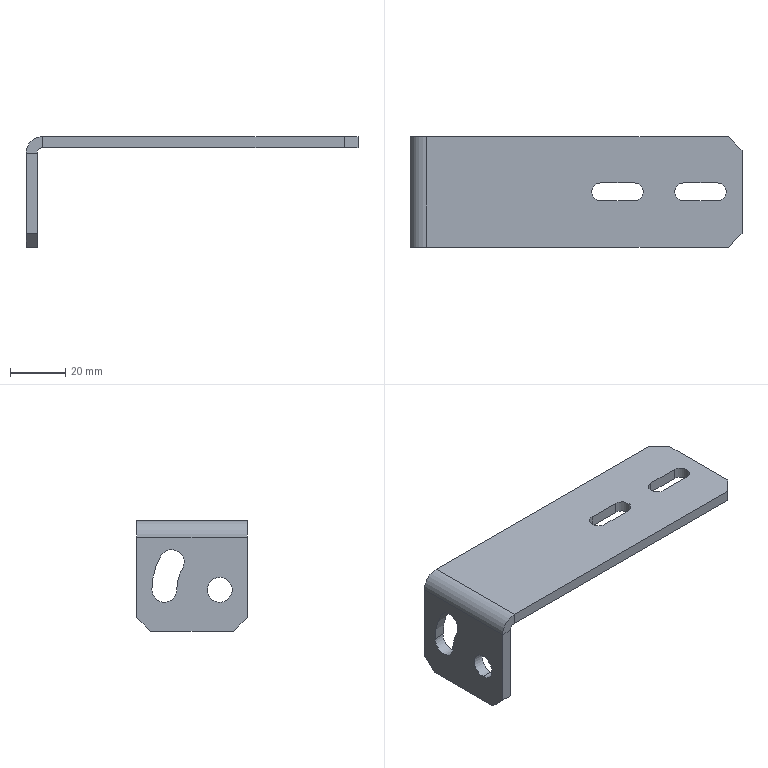Part | SolidWorks | features MoveFace 2, BaseBody 1, Chamfer 1, FlatPattern 1, SheetMetal 1, SolidToSheetMetal 1 | 1 solid | 33 faces | box 120 x 40 x 40 mm | volume 22710 mm3 | plane 20 | cylinder 13 | commonest cylinder face diameters 9 x5 6.5 x4 4 x1 12 x1 31 x1 49 x1
STEP:
#1=CARTESIAN_POINT('',(-52.,-10.,-20.5));
#2=VERTEX_POINT('',#1);
#3=CARTESIAN_POINT('',(-52.,-10.,-29.5));
#4=VERTEX_POINT('',#3);
#5=CARTESIAN_POINT('',(-52.,-10.,-25.));
#6=DIRECTION('',(1.,0.,0.));
#7=DIRECTION('',(0.,0.,-1.));
#8=AXIS2_PLACEMENT_3D('',#5,#6,#7);
#9=CIRCLE('',#8,4.5);
#10=EDGE_CURVE('',#2,#4,#9,.T.);
#11=ORIENTED_EDGE('',*,*,#10,.T.);
#12=CARTESIAN_POINT('',(-56.,-10.,-29.5));
#13=VERTEX_POINT('',#12);
#14=CARTESIAN_POINT('',(-52.,-10.,-29.5));
#15=DIRECTION('',(-1.,0.,0.));
#16=VECTOR('',#15,1000.);
#17=LINE('',#14,#16);
#18=EDGE_CURVE('',#4,#13,#17,.T.);
#19=ORIENTED_EDGE('',*,*,#18,.T.);
#20=CARTESIAN_POINT('',(-56.,-10.,-20.5));
#21=VERTEX_POINT('',#20);
#22=CARTESIAN_POINT('',(-56.,-10.,-25.));
#23=DIRECTION('',(1.,0.,0.));
#24=DIRECTION('',(0.,0.,-1.));
#25=AXIS2_PLACEMENT_3D('',#22,#23,#24);
#26=CIRCLE('',#25,4.5);
#27=EDGE_CURVE('',#21,#13,#26,.T.);
#28=ORIENTED_EDGE('',*,*,#27,.F.);
#29=CARTESIAN_POINT('',(-52.,-10.,-20.5));
#30=DIRECTION('',(-1.,0.,0.));
#31=VECTOR('',#30,1000.);
#32=LINE('',#29,#31);
#33=EDGE_CURVE('',#2,#21,#32,.T.);
#34=ORIENTED_EDGE('',*,*,#33,.F.);
#35=EDGE_LOOP('',(#11,#19,#28,#34));
#36=FACE_OUTER_BOUND('',#35,.T.);
#37=CARTESIAN_POINT('',(-52.,-10.,-25.));
#38=DIRECTION('',(-1.,0.,0.));
#39=DIRECTION('',(0.,0.,1.));
#40=AXIS2_PLACEMENT_3D('',#37,#38,#39);
#41=CYLINDRICAL_SURFACE('',#40,4.5);
#42=ADVANCED_FACE('',(#36),#41,.F.);
#43=CARTESIAN_POINT('',(-52.,11.218,-12.75));
#44=VERTEX_POINT('',#43);
#45=CARTESIAN_POINT('',(-52.,7.321,-10.5));
#46=VERTEX_POINT('',#45);
#47=CARTESIAN_POINT('',(-52.,7.321,-15.));
#48=DIRECTION('',(1.,0.,0.));
#49=DIRECTION('',(0.,0.,-1.));
#50=AXIS2_PLACEMENT_3D('',#47,#48,#49);
#51=CIRCLE('',#50,4.5);
#52=EDGE_CURVE('',#44,#46,#51,.T.);
#53=ORIENTED_EDGE('',*,*,#52,.T.);
#54=CARTESIAN_POINT('',(-56.,7.321,-10.5));
#55=VERTEX_POINT('',#54);
#56=CARTESIAN_POINT('',(-52.,7.321,-10.5));
#57=DIRECTION('',(-1.,0.,0.));
#58=VECTOR('',#57,1000.);
#59=LINE('',#56,#58);
#60=EDGE_CURVE('',#46,#55,#59,.T.);
#61=ORIENTED_EDGE('',*,*,#60,.T.);
#62=CARTESIAN_POINT('',(-56.,11.218,-12.75));
#63=VERTEX_POINT('',#62);
#64=CARTESIAN_POINT('',(-56.,7.321,-15.));
#65=DIRECTION('',(1.,0.,0.));
#66=DIRECTION('',(0.,0.,-1.));
#67=AXIS2_PLACEMENT_3D('',#64,#65,#66);
#68=CIRCLE('',#67,4.5);
#69=EDGE_CURVE('',#63,#55,#68,.T.);
#70=ORIENTED_EDGE('',*,*,#69,.F.);
#71=CARTESIAN_POINT('',(-52.,11.218,-12.75));
#72=DIRECTION('',(1.,0.,0.));
#73=VECTOR('',#72,1000.);
#74=LINE('',#71,#73);
#75=EDGE_CURVE('',#63,#44,#74,.T.);
#76=ORIENTED_EDGE('',*,*,#75,.T.);
#77=EDGE_LOOP('',(#53,#61,#70,#76));
#78=FACE_OUTER_BOUND('',#77,.T.);
#79=CARTESIAN_POINT('',(-52.,7.321,-15.));
#80=DIRECTION('',(-1.,0.,0.));
#81=DIRECTION('',(0.,0.,1.));
#82=AXIS2_PLACEMENT_3D('',#79,#80,#81);
#83=CYLINDRICAL_SURFACE('',#82,4.5);
#84=ADVANCED_FACE('',(#78),#83,.F.);
#85=CARTESIAN_POINT('',(13.,-3.25,0.));
#86=VERTEX_POINT('',#85);
#87=CARTESIAN_POINT('',(13.,-3.25,-4.));
#88=VERTEX_POINT('',#87);
#89=CARTESIAN_POINT('',(13.,-3.25,-4.));
#90=DIRECTION('',(0.,0.,-1.));
#91=VECTOR('',#90,1000.);
#92=LINE('',#89,#91);
#93=EDGE_CURVE('',#86,#88,#92,.T.);
#94=ORIENTED_EDGE('',*,*,#93,.F.);
#95=CARTESIAN_POINT('',(25.,-3.25,0.));
#96=VERTEX_POINT('',#95);
#97=CARTESIAN_POINT('',(13.,-3.25,0.));
#98=DIRECTION('',(1.,0.,0.));
#99=VECTOR('',#98,1000.);
#100=LINE('',#97,#99);
#101=EDGE_CURVE('',#86,#96,#100,.T.);
#102=ORIENTED_EDGE('',*,*,#101,.T.);
#103=CARTESIAN_POINT('',(25.,-3.25,-4.));
#104=VERTEX_POINT('',#103);
#105=CARTESIAN_POINT('',(25.,-3.25,-4.));
#106=DIRECTION('',(0.,0.,-1.));
#107=VECTOR('',#106,1000.);
#108=LINE('',#105,#107);
#109=EDGE_CURVE('',#96,#104,#108,.T.);
#110=ORIENTED_EDGE('',*,*,#109,.T.);
#111=CARTESIAN_POINT('',(13.,-3.25,-4.));
#112=DIRECTION('',(1.,0.,0.));
#113=VECTOR('',#112,1000.);
#114=LINE('',#111,#113);
#115=EDGE_CURVE('',#88,#104,#114,.T.);
#116=ORIENTED_EDGE('',*,*,#115,.F.);
#117=EDGE_LOOP('',(#94,#102,#110,#116));
#118=FACE_OUTER_BOUND('',#117,.T.);
#119=CARTESIAN_POINT('',(13.,-3.25,-4.));
#120=DIRECTION('',(0.,-1.,0.));
#121=DIRECTION('',(1.,0.,0.));
#122=AXIS2_PLACEMENT_3D('',#119,#120,#121);
#123=PLANE('',#122);
#124=ADVANCED_FACE('',(#118),#123,.F.);
#125=ORIENTED_EDGE('',*,*,#109,.F.);
#126=CARTESIAN_POINT('',(25.,3.25,0.));
#127=VERTEX_POINT('',#126);
#128=CARTESIAN_POINT('',(25.,0.,0.));
#129=DIRECTION('',(0.,0.,1.));
#130=DIRECTION('',(0.,-1.,0.));
#131=AXIS2_PLACEMENT_3D('',#128,#129,#130);
#132=CIRCLE('',#131,3.25);
#133=EDGE_CURVE('',#96,#127,#132,.T.);
#134=ORIENTED_EDGE('',*,*,#133,.T.);
#135=CARTESIAN_POINT('',(25.,3.25,-4.));
#136=VERTEX_POINT('',#135);
#137=CARTESIAN_POINT('',(25.,3.25,-4.));
#138=DIRECTION('',(0.,0.,-1.));
#139=VECTOR('',#138,1000.);
#140=LINE('',#137,#139);
#141=EDGE_CURVE('',#127,#136,#140,.T.);
#142=ORIENTED_EDGE('',*,*,#141,.T.);
#143=CARTESIAN_POINT('',(25.,0.,-4.));
#144=DIRECTION('',(0.,0.,1.));
#145=DIRECTION('',(1.,0.,0.));
#146=AXIS2_PLACEMENT_3D('',#143,#144,#145);
#147=CIRCLE('',#146,3.25);
#148=EDGE_CURVE('',#104,#136,#147,.T.);
#149=ORIENTED_EDGE('',*,*,#148,.F.);
#150=EDGE_LOOP('',(#125,#134,#142,#149));
#151=FACE_OUTER_BOUND('',#150,.T.);
#152=CARTESIAN_POINT('',(25.,0.,-4.));
#153=DIRECTION('',(0.,0.,1.));
#154=DIRECTION('',(0.,-1.,0.));
#155=AXIS2_PLACEMENT_3D('',#152,#153,#154);
#156=CYLINDRICAL_SURFACE('',#155,3.25);
#157=ADVANCED_FACE('',(#151),#156,.F.);
#158=ORIENTED_EDGE('',*,*,#141,.F.);
#159=CARTESIAN_POINT('',(13.,3.25,0.));
#160=VERTEX_POINT('',#159);
#161=CARTESIAN_POINT('',(13.,3.25,0.));
#162=DIRECTION('',(-1.,0.,0.));
#163=VECTOR('',#162,1000.);
#164=LINE('',#161,#163);
#165=EDGE_CURVE('',#127,#160,#164,.T.);
#166=ORIENTED_EDGE('',*,*,#165,.T.);
#167=CARTESIAN_POINT('',(13.,3.25,-4.));
#168=VERTEX_POINT('',#167);
#169=CARTESIAN_POINT('',(13.,3.25,-4.));
#170=DIRECTION('',(0.,0.,-1.));
#171=VECTOR('',#170,1000.);
#172=LINE('',#169,#171);
#173=EDGE_CURVE('',#160,#168,#172,.T.);
#174=ORIENTED_EDGE('',*,*,#173,.T.);
#175=CARTESIAN_POINT('',(13.,3.25,-4.));
#176=DIRECTION('',(-1.,0.,0.));
#177=VECTOR('',#176,1000.);
#178=LINE('',#175,#177);
#179=EDGE_CURVE('',#136,#168,#178,.T.);
#180=ORIENTED_EDGE('',*,*,#179,.F.);
#181=EDGE_LOOP('',(#158,#166,#174,#180));
#182=FACE_OUTER_BOUND('',#181,.T.);
#183=CARTESIAN_POINT('',(13.,3.25,-4.));
#184=DIRECTION('',(0.,1.,0.));
#185=DIRECTION('',(-1.,0.,0.));
#186=AXIS2_PLACEMENT_3D('',#183,#184,#185);
#187=PLANE('',#186);
#188=ADVANCED_FACE('',(#182),#187,.F.);
#189=CARTESIAN_POINT('',(43.,-3.25,0.));
#190=VERTEX_POINT('',#189);
#191=CARTESIAN_POINT('',(43.,-3.25,-4.));
#192=VERTEX_POINT('',#191);
#193=CARTESIAN_POINT('',(43.,-3.25,-4.));
#194=DIRECTION('',(0.,0.,-1.));
#195=VECTOR('',#194,1000.);
#196=LINE('',#193,#195);
#197=EDGE_CURVE('',#190,#192,#196,.T.);
#198=ORIENTED_EDGE('',*,*,#197,.F.);
#199=CARTESIAN_POINT('',(55.,-3.25,0.));
#200=VERTEX_POINT('',#199);
#201=CARTESIAN_POINT('',(13.,-3.25,0.));
#202=DIRECTION('',(1.,0.,0.));
#203=VECTOR('',#202,1000.);
#204=LINE('',#201,#203);
#205=EDGE_CURVE('',#190,#200,#204,.T.);
#206=ORIENTED_EDGE('',*,*,#205,.T.);
#207=CARTESIAN_POINT('',(55.,-3.25,-4.));
#208=VERTEX_POINT('',#207);
#209=CARTESIAN_POINT('',(55.,-3.25,-4.));
#210=DIRECTION('',(0.,0.,-1.));
#211=VECTOR('',#210,1000.);
#212=LINE('',#209,#211);
#213=EDGE_CURVE('',#200,#208,#212,.T.);
#214=ORIENTED_EDGE('',*,*,#213,.T.);
#215=CARTESIAN_POINT('',(13.,-3.25,-4.));
#216=DIRECTION('',(1.,0.,0.));
#217=VECTOR('',#216,1000.);
#218=LINE('',#215,#217);
#219=EDGE_CURVE('',#192,#208,#218,.T.);
#220=ORIENTED_EDGE('',*,*,#219,.F.);
#221=EDGE_LOOP('',(#198,#206,#214,#220));
#222=FACE_OUTER_BOUND('',#221,.T.);
#223=CARTESIAN_POINT('',(13.,-3.25,-4.));
#224=DIRECTION('',(0.,-1.,0.));
#225=DIRECTION('',(1.,0.,0.));
#226=AXIS2_PLACEMENT_3D('',#223,#224,#225);
#227=PLANE('',#226);
#228=ADVANCED_FACE('',(#222),#227,.F.);
#229=ORIENTED_EDGE('',*,*,#213,.F.);
#230=CARTESIAN_POINT('',(55.,3.25,0.));
#231=VERTEX_POINT('',#230);
#232=CARTESIAN_POINT('',(55.,0.,0.));
#233=DIRECTION('',(0.,0.,1.));
#234=DIRECTION('',(0.,-1.,0.));
#235=AXIS2_PLACEMENT_3D('',#232,#233,#234);
#236=CIRCLE('',#235,3.25);
#237=EDGE_CURVE('',#200,#231,#236,.T.);
#238=ORIENTED_EDGE('',*,*,#237,.T.);
#239=CARTESIAN_POINT('',(55.,3.25,-4.));
#240=VERTEX_POINT('',#239);
#241=CARTESIAN_POINT('',(55.,3.25,-4.));
#242=DIRECTION('',(0.,0.,-1.));
#243=VECTOR('',#242,1000.);
#244=LINE('',#241,#243);
#245=EDGE_CURVE('',#231,#240,#244,.T.);
#246=ORIENTED_EDGE('',*,*,#245,.T.);
#247=CARTESIAN_POINT('',(55.,0.,-4.));
#248=DIRECTION('',(0.,0.,1.));
#249=DIRECTION('',(1.,0.,0.));
#250=AXIS2_PLACEMENT_3D('',#247,#248,#249);
#251=CIRCLE('',#250,3.25);
#252=EDGE_CURVE('',#208,#240,#251,.T.);
#253=ORIENTED_EDGE('',*,*,#252,.F.);
#254=EDGE_LOOP('',(#229,#238,#246,#253));
#255=FACE_OUTER_BOUND('',#254,.T.);
#256=CARTESIAN_POINT('',(55.,0.,-4.));
#257=DIRECTION('',(0.,0.,1.));
#258=DIRECTION('',(0.,-1.,0.));
#259=AXIS2_PLACEMENT_3D('',#256,#257,#258);
#260=CYLINDRICAL_SURFACE('',#259,3.25);
#261=ADVANCED_FACE('',(#255),#260,.F.);
#262=ORIENTED_EDGE('',*,*,#245,.F.);
#263=CARTESIAN_POINT('',(43.,3.25,0.));
#264=VERTEX_POINT('',#263);
#265=CARTESIAN_POINT('',(13.,3.25,0.));
#266=DIRECTION('',(-1.,0.,0.));
#267=VECTOR('',#266,1000.);
#268=LINE('',#265,#267);
#269=EDGE_CURVE('',#231,#264,#268,.T.);
#270=ORIENTED_EDGE('',*,*,#269,.T.);
#271=CARTESIAN_POINT('',(43.,3.25,-4.));
#272=VERTEX_POINT('',#271);
#273=CARTESIAN_POINT('',(43.,3.25,-4.));
#274=DIRECTION('',(0.,0.,-1.));
#275=VECTOR('',#274,1000.);
#276=LINE('',#273,#275);
#277=EDGE_CURVE('',#264,#272,#276,.T.);
#278=ORIENTED_EDGE('',*,*,#277,.T.);
#279=CARTESIAN_POINT('',(13.,3.25,-4.));
#280=DIRECTION('',(-1.,0.,0.));
#281=VECTOR('',#280,1000.);
#282=LINE('',#279,#281);
#283=EDGE_CURVE('',#240,#272,#282,.T.);
#284=ORIENTED_EDGE('',*,*,#283,.F.);
#285=EDGE_LOOP('',(#262,#270,#278,#284));
#286=FACE_OUTER_BOUND('',#285,.T.);
#287=CARTESIAN_POINT('',(13.,3.25,-4.));
#288=DIRECTION('',(0.,1.,0.));
#289=DIRECTION('',(-1.,0.,0.));
#290=AXIS2_PLACEMENT_3D('',#287,#288,#289);
#291=PLANE('',#290);
#292=ADVANCED_FACE('',(#286),#291,.F.);
#293=ORIENTED_EDGE('',*,*,#60,.F.);
#294=CARTESIAN_POINT('',(-52.,3.423,-17.25));
#295=VERTEX_POINT('',#294);
#296=CARTESIAN_POINT('',(-52.,7.321,-15.));
#297=DIRECTION('',(1.,0.,0.));
#298=DIRECTION('',(0.,0.,-1.));
#299=AXIS2_PLACEMENT_3D('',#296,#297,#298);
#300=CIRCLE('',#299,4.5);
#301=EDGE_CURVE('',#46,#295,#300,.T.);
#302=ORIENTED_EDGE('',*,*,#301,.T.);
#303=CARTESIAN_POINT('',(-56.,3.423,-17.25));
#304=VERTEX_POINT('',#303);
#305=CARTESIAN_POINT('',(-52.,3.423,-17.25));
#306=DIRECTION('',(1.,0.,0.));
#307=VECTOR('',#306,1000.);
#308=LINE('',#305,#307);
#309=EDGE_CURVE('',#304,#295,#308,.T.);
#310=ORIENTED_EDGE('',*,*,#309,.F.);
#311=CARTESIAN_POINT('',(-56.,7.321,-15.));
#312=DIRECTION('',(1.,0.,0.));
#313=DIRECTION('',(0.,0.,-1.));
#314=AXIS2_PLACEMENT_3D('',#311,#312,#313);
#315=CIRCLE('',#314,4.5);
#316=EDGE_CURVE('',#55,#304,#315,.T.);
#317=ORIENTED_EDGE('',*,*,#316,.F.);
#318=EDGE_LOOP('',(#293,#302,#310,#317));
#319=FACE_OUTER_BOUND('',#318,.T.);
#320=CARTESIAN_POINT('',(-52.,7.321,-15.));
#321=DIRECTION('',(-1.,0.,0.));
#322=DIRECTION('',(0.,0.,1.));
#323=AXIS2_PLACEMENT_3D('',#320,#321,#322);
#324=CYLINDRICAL_SURFACE('',#323,4.5);
#325=ADVANCED_FACE('',(#319),#324,.F.);
#326=ORIENTED_EDGE('',*,*,#75,.F.);
#327=CARTESIAN_POINT('',(-56.,14.5,-25.));
#328=VERTEX_POINT('',#327);
#329=CARTESIAN_POINT('',(-56.,-10.,-25.));
#330=DIRECTION('',(1.,0.,0.));
#331=DIRECTION('',(0.,0.,-1.));
#332=AXIS2_PLACEMENT_3D('',#329,#330,#331);
#333=CIRCLE('',#332,24.5);
#334=EDGE_CURVE('',#328,#63,#333,.T.);
#335=ORIENTED_EDGE('',*,*,#334,.F.);
#336=CARTESIAN_POINT('',(-52.,14.5,-25.));
#337=VERTEX_POINT('',#336);
#338=CARTESIAN_POINT('',(-52.,14.5,-25.));
#339=DIRECTION('',(1.,0.,0.));
#340=VECTOR('',#339,1000.);
#341=LINE('',#338,#340);
#342=EDGE_CURVE('',#328,#337,#341,.T.);
#343=ORIENTED_EDGE('',*,*,#342,.T.);
#344=CARTESIAN_POINT('',(-52.,-10.,-25.));
#345=DIRECTION('',(1.,0.,0.));
#346=DIRECTION('',(0.,0.,-1.));
#347=AXIS2_PLACEMENT_3D('',#344,#345,#346);
#348=CIRCLE('',#347,24.5);
#349=EDGE_CURVE('',#337,#44,#348,.T.);
#350=ORIENTED_EDGE('',*,*,#349,.T.);
#351=EDGE_LOOP('',(#326,#335,#343,#350));
#352=FACE_OUTER_BOUND('',#351,.T.);
#353=CARTESIAN_POINT('',(-52.,-10.,-25.));
#354=DIRECTION('',(-1.,0.,0.));
#355=DIRECTION('',(0.,0.,1.));
#356=AXIS2_PLACEMENT_3D('',#353,#354,#355);
#357=CYLINDRICAL_SURFACE('',#356,24.5);
#358=ADVANCED_FACE('',(#352),#357,.F.);
#359=ORIENTED_EDGE('',*,*,#342,.F.);
#360=CARTESIAN_POINT('',(-56.,5.5,-25.));
#361=VERTEX_POINT('',#360);
#362=CARTESIAN_POINT('',(-56.,10.,-25.));
#363=DIRECTION('',(1.,0.,0.));
#364=DIRECTION('',(0.,0.,-1.));
#365=AXIS2_PLACEMENT_3D('',#362,#363,#364);
#366=CIRCLE('',#365,4.5);
#367=EDGE_CURVE('',#361,#328,#366,.T.);
#368=ORIENTED_EDGE('',*,*,#367,.F.);
#369=CARTESIAN_POINT('',(-52.,5.5,-25.));
#370=VERTEX_POINT('',#369);
#371=CARTESIAN_POINT('',(-52.,5.5,-25.));
#372=DIRECTION('',(1.,0.,0.));
#373=VECTOR('',#372,1000.);
#374=LINE('',#371,#373);
#375=EDGE_CURVE('',#361,#370,#374,.T.);
#376=ORIENTED_EDGE('',*,*,#375,.T.);
#377=CARTESIAN_POINT('',(-52.,10.,-25.));
#378=DIRECTION('',(1.,0.,0.));
#379=DIRECTION('',(0.,0.,-1.));
#380=AXIS2_PLACEMENT_3D('',#377,#378,#379);
#381=CIRCLE('',#380,4.5);
#382=EDGE_CURVE('',#370,#337,#381,.T.);
#383=ORIENTED_EDGE('',*,*,#382,.T.);
#384=EDGE_LOOP('',(#359,#368,#376,#383));
#385=FACE_OUTER_BOUND('',#384,.T.);
#386=CARTESIAN_POINT('',(-52.,10.,-25.));
#387=DIRECTION('',(-1.,0.,0.));
#388=DIRECTION('',(0.,0.,1.));
#389=AXIS2_PLACEMENT_3D('',#386,#387,#388);
#390=CYLINDRICAL_SURFACE('',#389,4.5);
#391=ADVANCED_FACE('',(#385),#390,.F.);
#392=CARTESIAN_POINT('',(-56.,-20.,-35.));
#393=VERTEX_POINT('',#392);
#394=CARTESIAN_POINT('',(-52.,-20.,-35.));
#395=VERTEX_POINT('',#394);
#396=CARTESIAN_POINT('',(-52.,-20.,-35.));
#397=DIRECTION('',(1.,0.,0.));
#398=VECTOR('',#397,1000.);
#399=LINE('',#396,#398);
#400=EDGE_CURVE('',#393,#395,#399,.T.);
#401=ORIENTED_EDGE('',*,*,#400,.F.);
#402=CARTESIAN_POINT('',(-56.,-15.,-40.));
#403=VERTEX_POINT('',#402);
#404=CARTESIAN_POINT('',(-56.,-20.,-35.));
#405=DIRECTION('',(0.,0.7071,-0.7071));
#406=VECTOR('',#405,1000.);
#407=LINE('',#404,#406);
#408=EDGE_CURVE('',#393,#403,#407,.T.);
#409=ORIENTED_EDGE('',*,*,#408,.T.);
#410=CARTESIAN_POINT('',(-52.,-15.,-40.));
#411=VERTEX_POINT('',#410);
#412=CARTESIAN_POINT('',(-52.,-15.,-40.));
#413=DIRECTION('',(1.,0.,0.));
#414=VECTOR('',#413,1000.);
#415=LINE('',#412,#414);
#416=EDGE_CURVE('',#403,#411,#415,.T.);
#417=ORIENTED_EDGE('',*,*,#416,.T.);
#418=CARTESIAN_POINT('',(-52.,-20.,-35.));
#419=DIRECTION('',(0.,0.7071,-0.7071));
#420=VECTOR('',#419,1000.);
#421=LINE('',#418,#420);
#422=EDGE_CURVE('',#395,#411,#421,.T.);
#423=ORIENTED_EDGE('',*,*,#422,.F.);
#424=EDGE_LOOP('',(#401,#409,#417,#423));
#425=FACE_OUTER_BOUND('',#424,.T.);
#426=CARTESIAN_POINT('',(-52.,-20.,-35.));
#427=DIRECTION('',(0.,0.7071,0.7071));
#428=DIRECTION('',(0.,0.7071,-0.7071));
#429=AXIS2_PLACEMENT_3D('',#426,#427,#428);
#430=PLANE('',#429);
#431=ADVANCED_FACE('',(#425),#430,.F.);
#432=ORIENTED_EDGE('',*,*,#416,.F.);
#433=CARTESIAN_POINT('',(-56.,15.,-40.));
#434=VERTEX_POINT('',#433);
#435=CARTESIAN_POINT('',(-56.,0.,-40.));
#436=DIRECTION('',(0.,1.,0.));
#437=VECTOR('',#436,1000.);
#438=LINE('',#435,#437);
#439=EDGE_CURVE('',#403,#434,#438,.T.);
#440=ORIENTED_EDGE('',*,*,#439,.T.);
#441=CARTESIAN_POINT('',(-52.,15.,-40.));
#442=VERTEX_POINT('',#441);
#443=CARTESIAN_POINT('',(-52.,15.,-40.));
#444=DIRECTION('',(1.,0.,0.));
#445=VECTOR('',#444,1000.);
#446=LINE('',#443,#445);
#447=EDGE_CURVE('',#434,#442,#446,.T.);
#448=ORIENTED_EDGE('',*,*,#447,.T.);
#449=CARTESIAN_POINT('',(-52.,0.,-40.));
#450=DIRECTION('',(0.,1.,0.));
#451=VECTOR('',#450,1000.);
#452=LINE('',#449,#451);
#453=EDGE_CURVE('',#411,#442,#452,.T.);
#454=ORIENTED_EDGE('',*,*,#453,.F.);
#455=EDGE_LOOP('',(#432,#440,#448,#454));
#456=FACE_OUTER_BOUND('',#455,.T.);
#457=CARTESIAN_POINT('',(-52.,0.,-40.));
#458=DIRECTION('',(0.,0.,1.));
#459=DIRECTION('',(0.,1.,0.));
#460=AXIS2_PLACEMENT_3D('',#457,#458,#459);
#461=PLANE('',#460);
#462=ADVANCED_FACE('',(#456),#461,.F.);
#463=ORIENTED_EDGE('',*,*,#447,.F.);
#464=CARTESIAN_POINT('',(-56.,20.,-35.));
#465=VERTEX_POINT('',#464);
#466=CARTESIAN_POINT('',(-56.,15.,-40.));
#467=DIRECTION('',(0.,0.7071,0.7071));
#468=VECTOR('',#467,1000.);
#469=LINE('',#466,#468);
#470=EDGE_CURVE('',#434,#465,#469,.T.);
#471=ORIENTED_EDGE('',*,*,#470,.T.);
#472=CARTESIAN_POINT('',(-52.,20.,-35.));
#473=VERTEX_POINT('',#472);
#474=CARTESIAN_POINT('',(-52.,20.,-35.));
#475=DIRECTION('',(1.,0.,0.));
#476=VECTOR('',#475,1000.);
#477=LINE('',#474,#476);
#478=EDGE_CURVE('',#465,#473,#477,.T.);
#479=ORIENTED_EDGE('',*,*,#478,.T.);
#480=CARTESIAN_POINT('',(-52.,15.,-40.));
#481=DIRECTION('',(0.,0.7071,0.7071));
#482=VECTOR('',#481,1000.);
#483=LINE('',#480,#482);
#484=EDGE_CURVE('',#442,#473,#483,.T.);
#485=ORIENTED_EDGE('',*,*,#484,.F.);
#486=EDGE_LOOP('',(#463,#471,#479,#485));
#487=FACE_OUTER_BOUND('',#486,.T.);
#488=CARTESIAN_POINT('',(-52.,15.,-40.));
#489=DIRECTION('',(0.,-0.7071,0.7071));
#490=DIRECTION('',(0.,0.7071,0.7071));
#491=AXIS2_PLACEMENT_3D('',#488,#489,#490);
#492=PLANE('',#491);
#493=ADVANCED_FACE('',(#487),#492,.F.);
#494=ORIENTED_EDGE('',*,*,#478,.F.);
#495=CARTESIAN_POINT('',(-56.,20.,-6.));
#496=VERTEX_POINT('',#495);
#497=CARTESIAN_POINT('',(-56.,20.,0.));
#498=DIRECTION('',(0.,0.,1.));
#499=VECTOR('',#498,1000.);
#500=LINE('',#497,#499);
#501=EDGE_CURVE('',#465,#496,#500,.T.);
#502=ORIENTED_EDGE('',*,*,#501,.T.);
#503=CARTESIAN_POINT('',(-52.,20.,-6.));
#504=VERTEX_POINT('',#503);
#505=CARTESIAN_POINT('',(-52.,20.,-6.));
#506=DIRECTION('',(1.,0.,0.));
#507=VECTOR('',#506,1000.);
#508=LINE('',#505,#507);
#509=EDGE_CURVE('',#496,#504,#508,.T.);
#510=ORIENTED_EDGE('',*,*,#509,.T.);
#511=CARTESIAN_POINT('',(-52.,20.,0.));
#512=DIRECTION('',(0.,0.,1.));
#513=VECTOR('',#512,1000.);
#514=LINE('',#511,#513);
#515=EDGE_CURVE('',#473,#504,#514,.T.);
#516=ORIENTED_EDGE('',*,*,#515,.F.);
#517=EDGE_LOOP('',(#494,#502,#510,#516));
#518=FACE_OUTER_BOUND('',#517,.T.);
#519=CARTESIAN_POINT('',(-52.,20.,0.));
#520=DIRECTION('',(0.,-1.,0.));
#521=DIRECTION('',(0.,0.,1.));
#522=AXIS2_PLACEMENT_3D('',#519,#520,#521);
#523=PLANE('',#522);
#524=ADVANCED_FACE('',(#518),#523,.F.);
#525=ORIENTED_EDGE('',*,*,#509,.F.);
#526=CARTESIAN_POINT('',(-50.,20.,0.));
#527=VERTEX_POINT('',#526);
#528=CARTESIAN_POINT('',(-50.,20.,-6.));
#529=DIRECTION('',(0.,1.,0.));
#530=DIRECTION('',(0.,0.,1.));
#531=AXIS2_PLACEMENT_3D('',#528,#529,#530);
#532=CIRCLE('',#531,6.);
#533=EDGE_CURVE('',#496,#527,#532,.T.);
#534=ORIENTED_EDGE('',*,*,#533,.T.);
#535=CARTESIAN_POINT('',(-50.,20.,-4.));
#536=VERTEX_POINT('',#535);
#537=CARTESIAN_POINT('',(-50.,20.,-4.));
#538=DIRECTION('',(0.,0.,-1.));
#539=VECTOR('',#538,1000.);
#540=LINE('',#537,#539);
#541=EDGE_CURVE('',#527,#536,#540,.T.);
#542=ORIENTED_EDGE('',*,*,#541,.T.);
#543=CARTESIAN_POINT('',(-50.,20.,-6.));
#544=DIRECTION('',(0.,1.,0.));
#545=DIRECTION('',(0.,0.,1.));
#546=AXIS2_PLACEMENT_3D('',#543,#544,#545);
#547=CIRCLE('',#546,2.);
#548=EDGE_CURVE('',#504,#536,#547,.T.);
#549=ORIENTED_EDGE('',*,*,#548,.F.);
#550=EDGE_LOOP('',(#525,#534,#542,#549));
#551=FACE_OUTER_BOUND('',#550,.T.);
#552=CARTESIAN_POINT('',(-50.,20.,-6.));
#553=DIRECTION('',(0.,-1.,0.));
#554=DIRECTION('',(0.,0.,-1.));
#555=AXIS2_PLACEMENT_3D('',#552,#553,#554);
#556=PLANE('',#555);
#557=ADVANCED_FACE('',(#551),#556,.F.);
#558=CARTESIAN_POINT('',(59.,20.,0.));
#559=VERTEX_POINT('',#558);
#560=CARTESIAN_POINT('',(0.,20.,0.));
#561=DIRECTION('',(-1.,0.,0.));
#562=VECTOR('',#561,1000.);
#563=LINE('',#560,#562);
#564=EDGE_CURVE('',#559,#527,#563,.T.);
#565=ORIENTED_EDGE('',*,*,#564,.F.);
#566=CARTESIAN_POINT('',(59.,20.,-4.));
#567=VERTEX_POINT('',#566);
#568=CARTESIAN_POINT('',(59.,20.,-4.));
#569=DIRECTION('',(0.,0.,-1.));
#570=VECTOR('',#569,1000.);
#571=LINE('',#568,#570);
#572=EDGE_CURVE('',#559,#567,#571,.T.);
#573=ORIENTED_EDGE('',*,*,#572,.T.);
#574=CARTESIAN_POINT('',(-56.,20.,-4.));
#575=DIRECTION('',(-1.,0.,0.));
#576=VECTOR('',#575,1000.);
#577=LINE('',#574,#576);
#578=EDGE_CURVE('',#567,#536,#577,.T.);
#579=ORIENTED_EDGE('',*,*,#578,.T.);
#580=ORIENTED_EDGE('',*,*,#541,.F.);
#581=EDGE_LOOP('',(#565,#573,#579,#580));
#582=FACE_OUTER_BOUND('',#581,.T.);
#583=CARTESIAN_POINT('',(-56.,20.,-4.));
#584=DIRECTION('',(0.,1.,0.));
#585=DIRECTION('',(-1.,0.,0.));
#586=AXIS2_PLACEMENT_3D('',#583,#584,#585);
#587=PLANE('',#586);
#588=ADVANCED_FACE('',(#582),#587,.T.);
#589=CARTESIAN_POINT('',(64.,-15.,0.));
#590=VERTEX_POINT('',#589);
#591=CARTESIAN_POINT('',(64.,15.,0.));
#592=VERTEX_POINT('',#591);
#593=CARTESIAN_POINT('',(64.,0.,0.));
#594=DIRECTION('',(0.,1.,0.));
#595=VECTOR('',#594,1000.);
#596=LINE('',#593,#595);
#597=EDGE_CURVE('',#590,#592,#596,.T.);
#598=ORIENTED_EDGE('',*,*,#597,.F.);
#599=CARTESIAN_POINT('',(64.,-15.,-4.));
#600=VERTEX_POINT('',#599);
#601=CARTESIAN_POINT('',(64.,-15.,-4.));
#602=DIRECTION('',(0.,0.,-1.));
#603=VECTOR('',#602,1000.);
#604=LINE('',#601,#603);
#605=EDGE_CURVE('',#590,#600,#604,.T.);
#606=ORIENTED_EDGE('',*,*,#605,.T.);
#607=CARTESIAN_POINT('',(64.,15.,-4.));
#608=VERTEX_POINT('',#607);
#609=CARTESIAN_POINT('',(64.,20.,-4.));
#610=DIRECTION('',(0.,1.,0.));
#611=VECTOR('',#610,1000.);
#612=LINE('',#609,#611);
#613=EDGE_CURVE('',#600,#608,#612,.T.);
#614=ORIENTED_EDGE('',*,*,#613,.T.);
#615=CARTESIAN_POINT('',(64.,15.,-4.));
#616=DIRECTION('',(0.,0.,1.));
#617=VECTOR('',#616,1000.);
#618=LINE('',#615,#617);
#619=EDGE_CURVE('',#608,#592,#618,.T.);
#620=ORIENTED_EDGE('',*,*,#619,.T.);
#621=EDGE_LOOP('',(#598,#606,#614,#620));
#622=FACE_OUTER_BOUND('',#621,.T.);
#623=CARTESIAN_POINT('',(64.,20.,-4.));
#624=DIRECTION('',(1.,0.,0.));
#625=DIRECTION('',(0.,1.,0.));
#626=AXIS2_PLACEMENT_3D('',#623,#624,#625);
#627=PLANE('',#626);
#628=ADVANCED_FACE('',(#622),#627,.T.);
#629=CARTESIAN_POINT('',(-50.,-20.,-4.));
#630=VERTEX_POINT('',#629);
#631=CARTESIAN_POINT('',(59.,-20.,-4.));
#632=VERTEX_POINT('',#631);
#633=CARTESIAN_POINT('',(-56.,-20.,-4.));
#634=DIRECTION('',(1.,0.,0.));
#635=VECTOR('',#634,1000.);
#636=LINE('',#633,#635);
#637=EDGE_CURVE('',#630,#632,#636,.T.);
#638=ORIENTED_EDGE('',*,*,#637,.T.);
#639=CARTESIAN_POINT('',(59.,-20.,0.));
#640=VERTEX_POINT('',#639);
#641=CARTESIAN_POINT('',(59.,-20.,-4.));
#642=DIRECTION('',(0.,0.,1.));
#643=VECTOR('',#642,1000.);
#644=LINE('',#641,#643);
#645=EDGE_CURVE('',#632,#640,#644,.T.);
#646=ORIENTED_EDGE('',*,*,#645,.T.);
#647=CARTESIAN_POINT('',(-50.,-20.,0.));
#648=VERTEX_POINT('',#647);
#649=CARTESIAN_POINT('',(0.,-20.,0.));
#650=DIRECTION('',(1.,0.,0.));
#651=VECTOR('',#650,1000.);
#652=LINE('',#649,#651);
#653=EDGE_CURVE('',#648,#640,#652,.T.);
#654=ORIENTED_EDGE('',*,*,#653,.F.);
#655=CARTESIAN_POINT('',(-50.,-20.,-4.));
#656=DIRECTION('',(0.,0.,-1.));
#657=VECTOR('',#656,1000.);
#658=LINE('',#655,#657);
#659=EDGE_CURVE('',#648,#630,#658,.T.);
#660=ORIENTED_EDGE('',*,*,#659,.T.);
#661=EDGE_LOOP('',(#638,#646,#654,#660));
#662=FACE_OUTER_BOUND('',#661,.T.);
#663=CARTESIAN_POINT('',(-56.,-20.,-4.));
#664=DIRECTION('',(0.,-1.,0.));
#665=DIRECTION('',(1.,0.,0.));
#666=AXIS2_PLACEMENT_3D('',#663,#664,#665);
#667=PLANE('',#666);
#668=ADVANCED_FACE('',(#662),#667,.T.);
#669=ORIENTED_EDGE('',*,*,#659,.F.);
#670=CARTESIAN_POINT('',(-56.,-20.,-6.));
#671=VERTEX_POINT('',#670);
#672=CARTESIAN_POINT('',(-50.,-20.,-6.));
#673=DIRECTION('',(0.,-1.,0.));
#674=DIRECTION('',(0.,0.,1.));
#675=AXIS2_PLACEMENT_3D('',#672,#673,#674);
#676=CIRCLE('',#675,6.);
#677=EDGE_CURVE('',#648,#671,#676,.T.);
#678=ORIENTED_EDGE('',*,*,#677,.T.);
#679=CARTESIAN_POINT('',(-52.,-20.,-6.));
#680=VERTEX_POINT('',#679);
#681=CARTESIAN_POINT('',(-52.,-20.,-6.));
#682=DIRECTION('',(1.,0.,0.));
#683=VECTOR('',#682,1000.);
#684=LINE('',#681,#683);
#685=EDGE_CURVE('',#671,#680,#684,.T.);
#686=ORIENTED_EDGE('',*,*,#685,.T.);
#687=CARTESIAN_POINT('',(-50.,-20.,-6.));
#688=DIRECTION('',(0.,-1.,0.));
#689=DIRECTION('',(0.,0.,1.));
#690=AXIS2_PLACEMENT_3D('',#687,#688,#689);
#691=CIRCLE('',#690,2.);
#692=EDGE_CURVE('',#630,#680,#691,.T.);
#693=ORIENTED_EDGE('',*,*,#692,.F.);
#694=EDGE_LOOP('',(#669,#678,#686,#693));
#695=FACE_OUTER_BOUND('',#694,.T.);
#696=CARTESIAN_POINT('',(-50.,-20.,-6.));
#697=DIRECTION('',(0.,1.,0.));
#698=DIRECTION('',(0.,0.,1.));
#699=AXIS2_PLACEMENT_3D('',#696,#697,#698);
#700=PLANE('',#699);
#701=ADVANCED_FACE('',(#695),#700,.F.);
#702=CARTESIAN_POINT('',(43.,0.,0.));
#703=DIRECTION('',(0.,0.,1.));
#704=DIRECTION('',(0.,-1.,0.));
#705=AXIS2_PLACEMENT_3D('',#702,#703,#704);
#706=CIRCLE('',#705,3.25);
#707=EDGE_CURVE('',#264,#190,#706,.T.);
#708=ORIENTED_EDGE('',*,*,#707,.T.);
#709=ORIENTED_EDGE('',*,*,#197,.T.);
#710=CARTESIAN_POINT('',(43.,0.,-4.));
#711=DIRECTION('',(0.,0.,1.));
#712=DIRECTION('',(1.,0.,0.));
#713=AXIS2_PLACEMENT_3D('',#710,#711,#712);
#714=CIRCLE('',#713,3.25);
#715=EDGE_CURVE('',#272,#192,#714,.T.);
#716=ORIENTED_EDGE('',*,*,#715,.F.);
#717=ORIENTED_EDGE('',*,*,#277,.F.);
#718=EDGE_LOOP('',(#708,#709,#716,#717));
#719=FACE_OUTER_BOUND('',#718,.T.);
#720=CARTESIAN_POINT('',(43.,0.,-4.));
#721=DIRECTION('',(0.,0.,1.));
#722=DIRECTION('',(0.,-1.,0.));
#723=AXIS2_PLACEMENT_3D('',#720,#721,#722);
#724=CYLINDRICAL_SURFACE('',#723,3.25);
#725=ADVANCED_FACE('',(#719),#724,.F.);
#726=CARTESIAN_POINT('',(13.,0.,0.));
#727=DIRECTION('',(0.,0.,1.));
#728=DIRECTION('',(0.,-1.,0.));
#729=AXIS2_PLACEMENT_3D('',#726,#727,#728);
#730=CIRCLE('',#729,3.25);
#731=EDGE_CURVE('',#160,#86,#730,.T.);
#732=ORIENTED_EDGE('',*,*,#731,.T.);
#733=ORIENTED_EDGE('',*,*,#93,.T.);
#734=CARTESIAN_POINT('',(13.,0.,-4.));
#735=DIRECTION('',(0.,0.,1.));
#736=DIRECTION('',(1.,0.,0.));
#737=AXIS2_PLACEMENT_3D('',#734,#735,#736);
#738=CIRCLE('',#737,3.25);
#739=EDGE_CURVE('',#168,#88,#738,.T.);
#740=ORIENTED_EDGE('',*,*,#739,.F.);
#741=ORIENTED_EDGE('',*,*,#173,.F.);
#742=EDGE_LOOP('',(#732,#733,#740,#741));
#743=FACE_OUTER_BOUND('',#742,.T.);
#744=CARTESIAN_POINT('',(13.,0.,-4.));
#745=DIRECTION('',(0.,0.,1.));
#746=DIRECTION('',(0.,-1.,0.));
#747=AXIS2_PLACEMENT_3D('',#744,#745,#746);
#748=CYLINDRICAL_SURFACE('',#747,3.25);
#749=ADVANCED_FACE('',(#743),#748,.F.);
#750=ORIENTED_EDGE('',*,*,#18,.F.);
#751=CARTESIAN_POINT('',(-52.,-10.,-25.));
#752=DIRECTION('',(1.,0.,0.));
#753=DIRECTION('',(0.,0.,-1.));
#754=AXIS2_PLACEMENT_3D('',#751,#752,#753);
#755=CIRCLE('',#754,4.5);
#756=EDGE_CURVE('',#4,#2,#755,.T.);
#757=ORIENTED_EDGE('',*,*,#756,.T.);
#758=ORIENTED_EDGE('',*,*,#33,.T.);
#759=CARTESIAN_POINT('',(-56.,-10.,-25.));
#760=DIRECTION('',(1.,0.,0.));
#761=DIRECTION('',(0.,0.,-1.));
#762=AXIS2_PLACEMENT_3D('',#759,#760,#761);
#763=CIRCLE('',#762,4.5);
#764=EDGE_CURVE('',#13,#21,#763,.T.);
#765=ORIENTED_EDGE('',*,*,#764,.F.);
#766=EDGE_LOOP('',(#750,#757,#758,#765));
#767=FACE_OUTER_BOUND('',#766,.T.);
#768=CARTESIAN_POINT('',(-52.,-10.,-25.));
#769=DIRECTION('',(-1.,0.,0.));
#770=DIRECTION('',(0.,0.,1.));
#771=AXIS2_PLACEMENT_3D('',#768,#769,#770);
#772=CYLINDRICAL_SURFACE('',#771,4.5);
#773=ADVANCED_FACE('',(#767),#772,.F.);
#774=CARTESIAN_POINT('',(-56.,-10.,-25.));
#775=DIRECTION('',(-1.,0.,0.));
#776=DIRECTION('',(0.,0.,1.));
#777=AXIS2_PLACEMENT_3D('',#774,#775,#776);
#778=CIRCLE('',#777,15.5);
#779=EDGE_CURVE('',#304,#361,#778,.T.);
#780=ORIENTED_EDGE('',*,*,#779,.F.);
#781=ORIENTED_EDGE('',*,*,#309,.T.);
#782=CARTESIAN_POINT('',(-52.,-10.,-25.));
#783=DIRECTION('',(-1.,0.,0.));
#784=DIRECTION('',(0.,0.,-1.));
#785=AXIS2_PLACEMENT_3D('',#782,#783,#784);
#786=CIRCLE('',#785,15.5);
#787=EDGE_CURVE('',#295,#370,#786,.T.);
#788=ORIENTED_EDGE('',*,*,#787,.T.);
#789=ORIENTED_EDGE('',*,*,#375,.F.);
#790=EDGE_LOOP('',(#780,#781,#788,#789));
#791=FACE_OUTER_BOUND('',#790,.T.);
#792=CARTESIAN_POINT('',(-52.,-10.,-25.));
#793=DIRECTION('',(-1.,0.,0.));
#794=DIRECTION('',(0.,0.,1.));
#795=AXIS2_PLACEMENT_3D('',#792,#793,#794);
#796=CYLINDRICAL_SURFACE('',#795,15.5);
#797=ADVANCED_FACE('',(#791),#796,.T.);
#798=CARTESIAN_POINT('',(-56.,-20.,0.));
#799=DIRECTION('',(0.,0.,-1.));
#800=VECTOR('',#799,1000.);
#801=LINE('',#798,#800);
#802=EDGE_CURVE('',#671,#393,#801,.T.);
#803=ORIENTED_EDGE('',*,*,#802,.T.);
#804=ORIENTED_EDGE('',*,*,#400,.T.);
#805=CARTESIAN_POINT('',(-52.,-20.,0.));
#806=DIRECTION('',(0.,0.,-1.));
#807=VECTOR('',#806,1000.);
#808=LINE('',#805,#807);
#809=EDGE_CURVE('',#680,#395,#808,.T.);
#810=ORIENTED_EDGE('',*,*,#809,.F.);
#811=ORIENTED_EDGE('',*,*,#685,.F.);
#812=EDGE_LOOP('',(#803,#804,#810,#811));
#813=FACE_OUTER_BOUND('',#812,.T.);
#814=CARTESIAN_POINT('',(-52.,-20.,0.));
#815=DIRECTION('',(0.,1.,0.));
#816=DIRECTION('',(0.,0.,-1.));
#817=AXIS2_PLACEMENT_3D('',#814,#815,#816);
#818=PLANE('',#817);
#819=ADVANCED_FACE('',(#813),#818,.F.);
#820=CARTESIAN_POINT('',(-50.,20.,-4.));
#821=DIRECTION('',(0.,-1.,0.));
#822=VECTOR('',#821,1000.);
#823=LINE('',#820,#822);
#824=EDGE_CURVE('',#536,#630,#823,.T.);
#825=ORIENTED_EDGE('',*,*,#824,.T.);
#826=ORIENTED_EDGE('',*,*,#692,.T.);
#827=CARTESIAN_POINT('',(-52.,-20.,-6.));
#828=DIRECTION('',(0.,1.,0.));
#829=VECTOR('',#828,1000.);
#830=LINE('',#827,#829);
#831=EDGE_CURVE('',#680,#504,#830,.T.);
#832=ORIENTED_EDGE('',*,*,#831,.T.);
#833=ORIENTED_EDGE('',*,*,#548,.T.);
#834=EDGE_LOOP('',(#825,#826,#832,#833));
#835=FACE_OUTER_BOUND('',#834,.T.);
#836=CARTESIAN_POINT('',(-50.,20.,-6.));
#837=DIRECTION('',(0.,1.,0.));
#838=DIRECTION('',(-1.,0.,0.));
#839=AXIS2_PLACEMENT_3D('',#836,#837,#838);
#840=CYLINDRICAL_SURFACE('',#839,2.);
#841=ADVANCED_FACE('',(#835),#840,.F.);
#842=ORIENTED_EDGE('',*,*,#10,.F.);
#843=ORIENTED_EDGE('',*,*,#756,.F.);
#844=EDGE_LOOP('',(#842,#843));
#845=FACE_BOUND('',#844,.T.);
#846=ORIENTED_EDGE('',*,*,#382,.F.);
#847=ORIENTED_EDGE('',*,*,#787,.F.);
#848=ORIENTED_EDGE('',*,*,#301,.F.);
#849=ORIENTED_EDGE('',*,*,#52,.F.);
#850=ORIENTED_EDGE('',*,*,#349,.F.);
#851=EDGE_LOOP('',(#846,#847,#848,#849,#850));
#852=FACE_BOUND('',#851,.T.);
#853=ORIENTED_EDGE('',*,*,#453,.T.);
#854=ORIENTED_EDGE('',*,*,#484,.T.);
#855=ORIENTED_EDGE('',*,*,#515,.T.);
#856=ORIENTED_EDGE('',*,*,#831,.F.);
#857=ORIENTED_EDGE('',*,*,#809,.T.);
#858=ORIENTED_EDGE('',*,*,#422,.T.);
#859=EDGE_LOOP('',(#853,#854,#855,#856,#857,#858));
#860=FACE_OUTER_BOUND('',#859,.T.);
#861=CARTESIAN_POINT('',(-52.,0.,0.));
#862=DIRECTION('',(-1.,0.,0.));
#863=DIRECTION('',(0.,1.,0.));
#864=AXIS2_PLACEMENT_3D('',#861,#862,#863);
#865=PLANE('',#864);
#866=ADVANCED_FACE('',(#845,#852,#860),#865,.F.);
#867=ORIENTED_EDGE('',*,*,#283,.T.);
#868=ORIENTED_EDGE('',*,*,#715,.T.);
#869=ORIENTED_EDGE('',*,*,#219,.T.);
#870=ORIENTED_EDGE('',*,*,#252,.T.);
#871=EDGE_LOOP('',(#867,#868,#869,#870));
#872=FACE_BOUND('',#871,.T.);
#873=ORIENTED_EDGE('',*,*,#179,.T.);
#874=ORIENTED_EDGE('',*,*,#739,.T.);
#875=ORIENTED_EDGE('',*,*,#115,.T.);
#876=ORIENTED_EDGE('',*,*,#148,.T.);
#877=EDGE_LOOP('',(#873,#874,#875,#876));
#878=FACE_BOUND('',#877,.T.);
#879=ORIENTED_EDGE('',*,*,#613,.F.);
#880=CARTESIAN_POINT('',(64.,-15.,-4.));
#881=DIRECTION('',(-0.7071,-0.7071,0.));
#882=VECTOR('',#881,1000.);
#883=LINE('',#880,#882);
#884=EDGE_CURVE('',#600,#632,#883,.T.);
#885=ORIENTED_EDGE('',*,*,#884,.T.);
#886=ORIENTED_EDGE('',*,*,#637,.F.);
#887=ORIENTED_EDGE('',*,*,#824,.F.);
#888=ORIENTED_EDGE('',*,*,#578,.F.);
#889=CARTESIAN_POINT('',(59.,20.,-4.));
#890=DIRECTION('',(0.7071,-0.7071,0.));
#891=VECTOR('',#890,1000.);
#892=LINE('',#889,#891);
#893=EDGE_CURVE('',#567,#608,#892,.T.);
#894=ORIENTED_EDGE('',*,*,#893,.T.);
#895=EDGE_LOOP('',(#879,#885,#886,#887,#888,#894));
#896=FACE_OUTER_BOUND('',#895,.T.);
#897=CARTESIAN_POINT('',(0.,0.,-4.));
#898=DIRECTION('',(0.,0.,1.));
#899=DIRECTION('',(0.,-1.,0.));
#900=AXIS2_PLACEMENT_3D('',#897,#898,#899);
#901=PLANE('',#900);
#902=ADVANCED_FACE('',(#872,#878,#896),#901,.F.);
#903=CARTESIAN_POINT('',(-50.,20.,0.));
#904=DIRECTION('',(0.,-1.,0.));
#905=VECTOR('',#904,1000.);
#906=LINE('',#903,#905);
#907=EDGE_CURVE('',#527,#648,#906,.T.);
#908=ORIENTED_EDGE('',*,*,#907,.F.);
#909=ORIENTED_EDGE('',*,*,#533,.F.);
#910=CARTESIAN_POINT('',(-56.,20.,-6.));
#911=DIRECTION('',(0.,1.,0.));
#912=VECTOR('',#911,1000.);
#913=LINE('',#910,#912);
#914=EDGE_CURVE('',#671,#496,#913,.T.);
#915=ORIENTED_EDGE('',*,*,#914,.F.);
#916=ORIENTED_EDGE('',*,*,#677,.F.);
#917=EDGE_LOOP('',(#908,#909,#915,#916));
#918=FACE_OUTER_BOUND('',#917,.T.);
#919=CARTESIAN_POINT('',(-50.,20.,-6.));
#920=DIRECTION('',(0.,1.,0.));
#921=DIRECTION('',(-1.,0.,0.));
#922=AXIS2_PLACEMENT_3D('',#919,#920,#921);
#923=CYLINDRICAL_SURFACE('',#922,6.);
#924=ADVANCED_FACE('',(#918),#923,.T.);
#925=ORIENTED_EDGE('',*,*,#27,.T.);
#926=ORIENTED_EDGE('',*,*,#764,.T.);
#927=EDGE_LOOP('',(#925,#926));
#928=FACE_BOUND('',#927,.T.);
#929=ORIENTED_EDGE('',*,*,#367,.T.);
#930=ORIENTED_EDGE('',*,*,#334,.T.);
#931=ORIENTED_EDGE('',*,*,#69,.T.);
#932=ORIENTED_EDGE('',*,*,#316,.T.);
#933=ORIENTED_EDGE('',*,*,#779,.T.);
#934=EDGE_LOOP('',(#929,#930,#931,#932,#933));
#935=FACE_BOUND('',#934,.T.);
#936=ORIENTED_EDGE('',*,*,#439,.F.);
#937=ORIENTED_EDGE('',*,*,#408,.F.);
#938=ORIENTED_EDGE('',*,*,#802,.F.);
#939=ORIENTED_EDGE('',*,*,#914,.T.);
#940=ORIENTED_EDGE('',*,*,#501,.F.);
#941=ORIENTED_EDGE('',*,*,#470,.F.);
#942=EDGE_LOOP('',(#936,#937,#938,#939,#940,#941));
#943=FACE_OUTER_BOUND('',#942,.T.);
#944=CARTESIAN_POINT('',(-56.,0.,0.));
#945=DIRECTION('',(-1.,0.,0.));
#946=DIRECTION('',(0.,1.,0.));
#947=AXIS2_PLACEMENT_3D('',#944,#945,#946);
#948=PLANE('',#947);
#949=ADVANCED_FACE('',(#928,#935,#943),#948,.T.);
#950=ORIENTED_EDGE('',*,*,#269,.F.);
#951=ORIENTED_EDGE('',*,*,#237,.F.);
#952=ORIENTED_EDGE('',*,*,#205,.F.);
#953=ORIENTED_EDGE('',*,*,#707,.F.);
#954=EDGE_LOOP('',(#950,#951,#952,#953));
#955=FACE_BOUND('',#954,.T.);
#956=ORIENTED_EDGE('',*,*,#165,.F.);
#957=ORIENTED_EDGE('',*,*,#133,.F.);
#958=ORIENTED_EDGE('',*,*,#101,.F.);
#959=ORIENTED_EDGE('',*,*,#731,.F.);
#960=EDGE_LOOP('',(#956,#957,#958,#959));
#961=FACE_BOUND('',#960,.T.);
#962=ORIENTED_EDGE('',*,*,#653,.T.);
#963=CARTESIAN_POINT('',(39.5,-39.5,0.));
#964=DIRECTION('',(0.7071,0.7071,0.));
#965=VECTOR('',#964,1000.);
#966=LINE('',#963,#965);
#967=EDGE_CURVE('',#640,#590,#966,.T.);
#968=ORIENTED_EDGE('',*,*,#967,.T.);
#969=ORIENTED_EDGE('',*,*,#597,.T.);
#970=CARTESIAN_POINT('',(39.5,39.5,0.));
#971=DIRECTION('',(-0.7071,0.7071,0.));
#972=VECTOR('',#971,1000.);
#973=LINE('',#970,#972);
#974=EDGE_CURVE('',#592,#559,#973,.T.);
#975=ORIENTED_EDGE('',*,*,#974,.T.);
#976=ORIENTED_EDGE('',*,*,#564,.T.);
#977=ORIENTED_EDGE('',*,*,#907,.T.);
#978=EDGE_LOOP('',(#962,#968,#969,#975,#976,#977));
#979=FACE_OUTER_BOUND('',#978,.T.);
#980=CARTESIAN_POINT('',(0.,0.,0.));
#981=DIRECTION('',(0.,0.,1.));
#982=DIRECTION('',(0.,-1.,0.));
#983=AXIS2_PLACEMENT_3D('',#980,#981,#982);
#984=PLANE('',#983);
#985=ADVANCED_FACE('',(#955,#961,#979),#984,.T.);
#986=ORIENTED_EDGE('',*,*,#967,.F.);
#987=ORIENTED_EDGE('',*,*,#645,.F.);
#988=ORIENTED_EDGE('',*,*,#884,.F.);
#989=ORIENTED_EDGE('',*,*,#605,.F.);
#990=EDGE_LOOP('',(#986,#987,#988,#989));
#991=FACE_OUTER_BOUND('',#990,.T.);
#992=CARTESIAN_POINT('',(64.,-15.,-4.));
#993=DIRECTION('',(-0.7071,0.7071,0.));
#994=DIRECTION('',(0.,0.,-1.));
#995=AXIS2_PLACEMENT_3D('',#992,#993,#994);
#996=PLANE('',#995);
#997=ADVANCED_FACE('',(#991),#996,.F.);
#998=ORIENTED_EDGE('',*,*,#974,.F.);
#999=ORIENTED_EDGE('',*,*,#619,.F.);
#1000=ORIENTED_EDGE('',*,*,#893,.F.);
#1001=ORIENTED_EDGE('',*,*,#572,.F.);
#1002=EDGE_LOOP('',(#998,#999,#1000,#1001));
#1003=FACE_OUTER_BOUND('',#1002,.T.);
#1004=CARTESIAN_POINT('',(59.,20.,-4.));
#1005=DIRECTION('',(-0.7071,-0.7071,0.));
#1006=DIRECTION('',(0.,0.,-1.));
#1007=AXIS2_PLACEMENT_3D('',#1004,#1005,#1006);
#1008=PLANE('',#1007);
#1009=ADVANCED_FACE('',(#1003),#1008,.F.);
#1010=CLOSED_SHELL('',(#42,#84,#124,#157,#188,#228,#261,#292,#325,#358,#391,#431,#462,#493,#524,#557,#588,#628,#668,#701,#725,#749,#773,#797,#819,#841,#866,#902,#924,#949,#985,#997,#1009));
#1011=MANIFOLD_SOLID_BREP('',#1010);
#1012=CARTESIAN_POINT('',(0.,0.,0.));
#1013=DIRECTION('',(0.,0.,1.));
#1014=DIRECTION('',(1.,0.,0.));
#1015=AXIS2_PLACEMENT_3D('',#1012,#1013,#1014);
#1016=(LENGTH_UNIT()NAMED_UNIT(*)SI_UNIT(.MILLI.,.METRE.));
#1017=UNCERTAINTY_MEASURE_WITH_UNIT(LENGTH_MEASURE(0.00001),#1016,'','');
#1018=(NAMED_UNIT(*)PLANE_ANGLE_UNIT()SI_UNIT($,.RADIAN.));
#1019=(NAMED_UNIT(*)SI_UNIT($,.STERADIAN.)SOLID_ANGLE_UNIT());
#1020=(GEOMETRIC_REPRESENTATION_CONTEXT(3)GLOBAL_UNCERTAINTY_ASSIGNED_CONTEXT((#1017))GLOBAL_UNIT_ASSIGNED_CONTEXT((#1016,#1018,#1019))REPRESENTATION_CONTEXT('',''));
#1021=ADVANCED_BREP_SHAPE_REPRESENTATION('',(#1011,#1015),#1020);